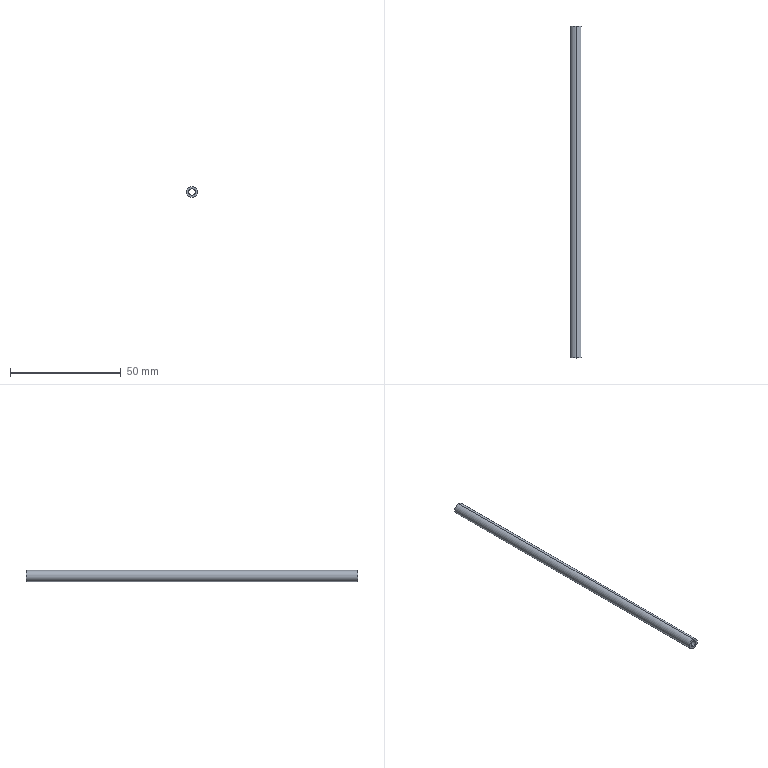Part | SolidWorks | features Extrusion 1 | 1 solid | 6 faces | box 5 x 150 x 5 mm | volume 1885 mm3 | cylinder 4 | plane 2 | commonest cylinder face diameters 3 x2 5 x2
STEP:
#1=CARTESIAN_POINT('',(0.,150.,-1.5));
#2=VERTEX_POINT('',#1);
#3=CARTESIAN_POINT('',(0.,150.,1.5));
#4=VERTEX_POINT('',#3);
#5=CARTESIAN_POINT('',(0.,150.,0.));
#6=DIRECTION('',(0.,1.,0.));
#7=DIRECTION('',(0.,0.,1.));
#8=AXIS2_PLACEMENT_3D('',#5,#6,#7);
#9=CIRCLE('',#8,1.5);
#10=EDGE_CURVE('',#2,#4,#9,.T.);
#11=ORIENTED_EDGE('',*,*,#10,.T.);
#12=CARTESIAN_POINT('',(0.,0.,1.5));
#13=VERTEX_POINT('',#12);
#14=CARTESIAN_POINT('',(0.,150.,1.5));
#15=DIRECTION('',(0.,-1.,0.));
#16=VECTOR('',#15,1000.);
#17=LINE('',#14,#16);
#18=EDGE_CURVE('',#4,#13,#17,.T.);
#19=ORIENTED_EDGE('',*,*,#18,.T.);
#20=CARTESIAN_POINT('',(0.,0.,-1.5));
#21=VERTEX_POINT('',#20);
#22=CARTESIAN_POINT('',(0.,0.,0.));
#23=DIRECTION('',(0.,1.,0.));
#24=DIRECTION('',(0.,0.,1.));
#25=AXIS2_PLACEMENT_3D('',#22,#23,#24);
#26=CIRCLE('',#25,1.5);
#27=EDGE_CURVE('',#21,#13,#26,.T.);
#28=ORIENTED_EDGE('',*,*,#27,.F.);
#29=CARTESIAN_POINT('',(0.,150.,-1.5));
#30=DIRECTION('',(0.,-1.,0.));
#31=VECTOR('',#30,1000.);
#32=LINE('',#29,#31);
#33=EDGE_CURVE('',#2,#21,#32,.T.);
#34=ORIENTED_EDGE('',*,*,#33,.F.);
#35=EDGE_LOOP('',(#11,#19,#28,#34));
#36=FACE_OUTER_BOUND('',#35,.T.);
#37=CARTESIAN_POINT('',(0.,150.,0.));
#38=DIRECTION('',(0.,-1.,0.));
#39=DIRECTION('',(0.,0.,-1.));
#40=AXIS2_PLACEMENT_3D('',#37,#38,#39);
#41=CYLINDRICAL_SURFACE('',#40,1.5);
#42=ADVANCED_FACE('',(#36),#41,.F.);
#43=CARTESIAN_POINT('',(0.,150.,2.5));
#44=VERTEX_POINT('',#43);
#45=CARTESIAN_POINT('',(0.,150.,-2.5));
#46=VERTEX_POINT('',#45);
#47=CARTESIAN_POINT('',(0.,150.,0.));
#48=DIRECTION('',(0.,1.,0.));
#49=DIRECTION('',(0.,0.,1.));
#50=AXIS2_PLACEMENT_3D('',#47,#48,#49);
#51=CIRCLE('',#50,2.5);
#52=EDGE_CURVE('',#44,#46,#51,.T.);
#53=ORIENTED_EDGE('',*,*,#52,.F.);
#54=CARTESIAN_POINT('',(0.,0.,2.5));
#55=VERTEX_POINT('',#54);
#56=CARTESIAN_POINT('',(0.,150.,2.5));
#57=DIRECTION('',(0.,-1.,0.));
#58=VECTOR('',#57,1000.);
#59=LINE('',#56,#58);
#60=EDGE_CURVE('',#44,#55,#59,.T.);
#61=ORIENTED_EDGE('',*,*,#60,.T.);
#62=CARTESIAN_POINT('',(0.,0.,-2.5));
#63=VERTEX_POINT('',#62);
#64=CARTESIAN_POINT('',(0.,0.,0.));
#65=DIRECTION('',(0.,1.,0.));
#66=DIRECTION('',(0.,0.,1.));
#67=AXIS2_PLACEMENT_3D('',#64,#65,#66);
#68=CIRCLE('',#67,2.5);
#69=EDGE_CURVE('',#55,#63,#68,.T.);
#70=ORIENTED_EDGE('',*,*,#69,.T.);
#71=CARTESIAN_POINT('',(0.,150.,-2.5));
#72=DIRECTION('',(0.,-1.,0.));
#73=VECTOR('',#72,1000.);
#74=LINE('',#71,#73);
#75=EDGE_CURVE('',#46,#63,#74,.T.);
#76=ORIENTED_EDGE('',*,*,#75,.F.);
#77=EDGE_LOOP('',(#53,#61,#70,#76));
#78=FACE_OUTER_BOUND('',#77,.T.);
#79=CARTESIAN_POINT('',(0.,150.,0.));
#80=DIRECTION('',(0.,-1.,0.));
#81=DIRECTION('',(0.,0.,-1.));
#82=AXIS2_PLACEMENT_3D('',#79,#80,#81);
#83=CYLINDRICAL_SURFACE('',#82,2.5);
#84=ADVANCED_FACE('',(#78),#83,.T.);
#85=CARTESIAN_POINT('',(0.,150.,0.));
#86=DIRECTION('',(0.,1.,0.));
#87=DIRECTION('',(0.,0.,1.));
#88=AXIS2_PLACEMENT_3D('',#85,#86,#87);
#89=CIRCLE('',#88,2.5);
#90=EDGE_CURVE('',#46,#44,#89,.T.);
#91=ORIENTED_EDGE('',*,*,#90,.T.);
#92=ORIENTED_EDGE('',*,*,#52,.T.);
#93=EDGE_LOOP('',(#91,#92));
#94=FACE_OUTER_BOUND('',#93,.T.);
#95=ORIENTED_EDGE('',*,*,#10,.F.);
#96=CARTESIAN_POINT('',(0.,150.,0.));
#97=DIRECTION('',(0.,1.,0.));
#98=DIRECTION('',(0.,0.,1.));
#99=AXIS2_PLACEMENT_3D('',#96,#97,#98);
#100=CIRCLE('',#99,1.5);
#101=EDGE_CURVE('',#4,#2,#100,.T.);
#102=ORIENTED_EDGE('',*,*,#101,.F.);
#103=EDGE_LOOP('',(#95,#102));
#104=FACE_BOUND('',#103,.T.);
#105=CARTESIAN_POINT('',(0.,150.,0.));
#106=DIRECTION('',(0.,1.,0.));
#107=DIRECTION('',(0.,0.,1.));
#108=AXIS2_PLACEMENT_3D('',#105,#106,#107);
#109=PLANE('',#108);
#110=ADVANCED_FACE('',(#94,#104),#109,.T.);
#111=CARTESIAN_POINT('',(0.,0.,0.));
#112=DIRECTION('',(0.,1.,0.));
#113=DIRECTION('',(0.,0.,1.));
#114=AXIS2_PLACEMENT_3D('',#111,#112,#113);
#115=CIRCLE('',#114,2.5);
#116=EDGE_CURVE('',#63,#55,#115,.T.);
#117=ORIENTED_EDGE('',*,*,#116,.F.);
#118=ORIENTED_EDGE('',*,*,#69,.F.);
#119=EDGE_LOOP('',(#117,#118));
#120=FACE_OUTER_BOUND('',#119,.T.);
#121=ORIENTED_EDGE('',*,*,#27,.T.);
#122=CARTESIAN_POINT('',(0.,0.,0.));
#123=DIRECTION('',(0.,1.,0.));
#124=DIRECTION('',(0.,0.,1.));
#125=AXIS2_PLACEMENT_3D('',#122,#123,#124);
#126=CIRCLE('',#125,1.5);
#127=EDGE_CURVE('',#13,#21,#126,.T.);
#128=ORIENTED_EDGE('',*,*,#127,.T.);
#129=EDGE_LOOP('',(#121,#128));
#130=FACE_BOUND('',#129,.T.);
#131=CARTESIAN_POINT('',(0.,0.,0.));
#132=DIRECTION('',(0.,1.,0.));
#133=DIRECTION('',(0.,0.,1.));
#134=AXIS2_PLACEMENT_3D('',#131,#132,#133);
#135=PLANE('',#134);
#136=ADVANCED_FACE('',(#120,#130),#135,.F.);
#137=ORIENTED_EDGE('',*,*,#60,.F.);
#138=ORIENTED_EDGE('',*,*,#90,.F.);
#139=ORIENTED_EDGE('',*,*,#75,.T.);
#140=ORIENTED_EDGE('',*,*,#116,.T.);
#141=EDGE_LOOP('',(#137,#138,#139,#140));
#142=FACE_OUTER_BOUND('',#141,.T.);
#143=CARTESIAN_POINT('',(0.,150.,0.));
#144=DIRECTION('',(0.,-1.,0.));
#145=DIRECTION('',(0.,0.,-1.));
#146=AXIS2_PLACEMENT_3D('',#143,#144,#145);
#147=CYLINDRICAL_SURFACE('',#146,2.5);
#148=ADVANCED_FACE('',(#142),#147,.T.);
#149=ORIENTED_EDGE('',*,*,#18,.F.);
#150=ORIENTED_EDGE('',*,*,#101,.T.);
#151=ORIENTED_EDGE('',*,*,#33,.T.);
#152=ORIENTED_EDGE('',*,*,#127,.F.);
#153=EDGE_LOOP('',(#149,#150,#151,#152));
#154=FACE_OUTER_BOUND('',#153,.T.);
#155=CARTESIAN_POINT('',(0.,150.,0.));
#156=DIRECTION('',(0.,-1.,0.));
#157=DIRECTION('',(0.,0.,-1.));
#158=AXIS2_PLACEMENT_3D('',#155,#156,#157);
#159=CYLINDRICAL_SURFACE('',#158,1.5);
#160=ADVANCED_FACE('',(#154),#159,.F.);
#161=CLOSED_SHELL('',(#42,#84,#110,#136,#148,#160));
#162=MANIFOLD_SOLID_BREP('',#161);
#163=CARTESIAN_POINT('',(0.,0.,0.));
#164=DIRECTION('',(0.,0.,1.));
#165=DIRECTION('',(1.,0.,0.));
#166=AXIS2_PLACEMENT_3D('',#163,#164,#165);
#167=(LENGTH_UNIT()NAMED_UNIT(*)SI_UNIT(.MILLI.,.METRE.));
#168=UNCERTAINTY_MEASURE_WITH_UNIT(LENGTH_MEASURE(0.00001),#167,'','');
#169=(NAMED_UNIT(*)PLANE_ANGLE_UNIT()SI_UNIT($,.RADIAN.));
#170=(NAMED_UNIT(*)SI_UNIT($,.STERADIAN.)SOLID_ANGLE_UNIT());
#171=(GEOMETRIC_REPRESENTATION_CONTEXT(3)GLOBAL_UNCERTAINTY_ASSIGNED_CONTEXT((#168))GLOBAL_UNIT_ASSIGNED_CONTEXT((#167,#169,#170))REPRESENTATION_CONTEXT('',''));
#172=ADVANCED_BREP_SHAPE_REPRESENTATION('',(#162,#166),#171);